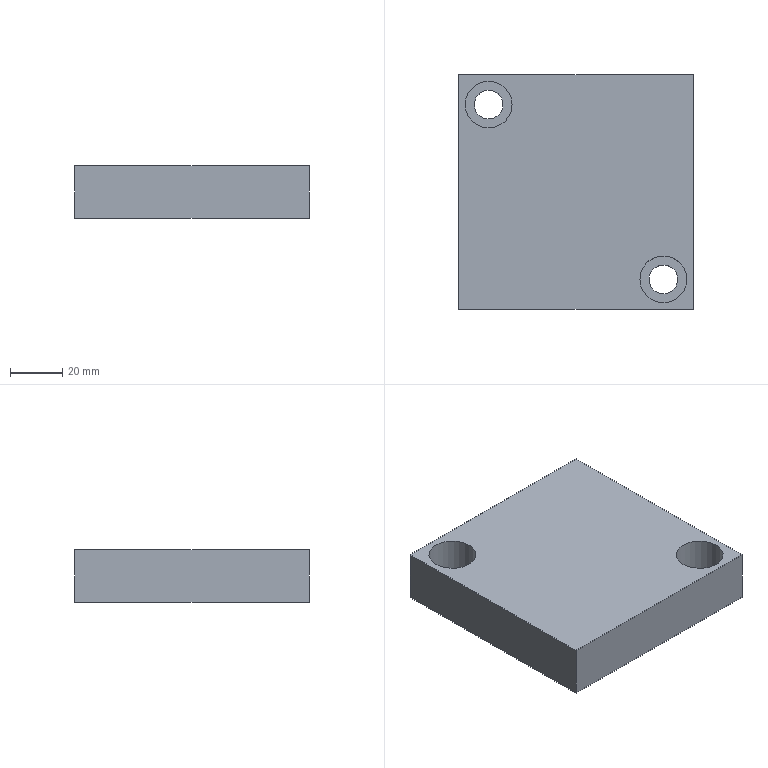Part | NX | features solid 2 | 1 solid | 12 faces | box 90 x 90 x 20 mm | volume 154053 mm3 | plane 8 | cylinder 4 | commonest cylinder face diameters 11 x2 18 x2
STEP:
#1=CARTESIAN_POINT('',(-2175.,-680.,-16.));
#2=VERTEX_POINT('',#1);
#3=CARTESIAN_POINT('',(-2175.,-680.,-36.));
#4=VERTEX_POINT('',#3);
#5=CARTESIAN_POINT('',(-2175.,-680.,-16.));
#6=DIRECTION('',(0.,0.,-1.));
#7=VECTOR('',#6,1000.);
#8=LINE('',#5,#7);
#9=EDGE_CURVE('',#2,#4,#8,.T.);
#10=ORIENTED_EDGE('',*,*,#9,.T.);
#11=CARTESIAN_POINT('',(-2085.,-680.,-36.));
#12=VERTEX_POINT('',#11);
#13=CARTESIAN_POINT('',(-2094.5,-680.,-36.));
#14=DIRECTION('',(-1.,0.,0.));
#15=VECTOR('',#14,1000.);
#16=LINE('',#13,#15);
#17=EDGE_CURVE('',#12,#4,#16,.T.);
#18=ORIENTED_EDGE('',*,*,#17,.F.);
#19=CARTESIAN_POINT('',(-2085.,-680.,-16.));
#20=VERTEX_POINT('',#19);
#21=CARTESIAN_POINT('',(-2085.,-680.,-16.));
#22=DIRECTION('',(0.,0.,1.));
#23=VECTOR('',#22,1000.);
#24=LINE('',#21,#23);
#25=EDGE_CURVE('',#20,#12,#24,.F.);
#26=ORIENTED_EDGE('',*,*,#25,.F.);
#27=CARTESIAN_POINT('',(-2094.5,-680.,-16.));
#28=DIRECTION('',(-1.,0.,0.));
#29=VECTOR('',#28,1000.);
#30=LINE('',#27,#29);
#31=EDGE_CURVE('',#20,#2,#30,.T.);
#32=ORIENTED_EDGE('',*,*,#31,.T.);
#33=EDGE_LOOP('',(#10,#18,#26,#32));
#34=FACE_BOUND('',#33,.T.);
#35=CARTESIAN_POINT('',(-2094.5,-680.,-16.));
#36=DIRECTION('',(0.,-1.,0.));
#37=DIRECTION('',(-1.,0.,0.));
#38=AXIS2_PLACEMENT_3D('',#35,#36,#37);
#39=PLANE('',#38);
#40=ADVANCED_FACE('',(#34),#39,.T.);
#41=ORIENTED_EDGE('',*,*,#25,.T.);
#42=CARTESIAN_POINT('',(-2085.,-590.,-36.));
#43=VERTEX_POINT('',#42);
#44=CARTESIAN_POINT('',(-2085.,-670.5,-36.));
#45=DIRECTION('',(0.,-1.,0.));
#46=VECTOR('',#45,1000.);
#47=LINE('',#44,#46);
#48=EDGE_CURVE('',#12,#43,#47,.F.);
#49=ORIENTED_EDGE('',*,*,#48,.T.);
#50=CARTESIAN_POINT('',(-2085.,-590.,-16.));
#51=VERTEX_POINT('',#50);
#52=CARTESIAN_POINT('',(-2085.,-590.,-16.));
#53=DIRECTION('',(0.,0.,-1.));
#54=VECTOR('',#53,1000.);
#55=LINE('',#52,#54);
#56=EDGE_CURVE('',#51,#43,#55,.T.);
#57=ORIENTED_EDGE('',*,*,#56,.F.);
#58=CARTESIAN_POINT('',(-2085.,-670.5,-16.));
#59=DIRECTION('',(0.,-1.,0.));
#60=VECTOR('',#59,1000.);
#61=LINE('',#58,#60);
#62=EDGE_CURVE('',#20,#51,#61,.F.);
#63=ORIENTED_EDGE('',*,*,#62,.F.);
#64=EDGE_LOOP('',(#41,#49,#57,#63));
#65=FACE_BOUND('',#64,.T.);
#66=CARTESIAN_POINT('',(-2085.,-670.5,-16.));
#67=DIRECTION('',(-1.,0.,0.));
#68=DIRECTION('',(0.,1.,0.));
#69=AXIS2_PLACEMENT_3D('',#66,#67,#68);
#70=PLANE('',#69);
#71=ADVANCED_FACE('',(#65),#70,.F.);
#72=ORIENTED_EDGE('',*,*,#56,.T.);
#73=CARTESIAN_POINT('',(-2175.,-590.,-36.));
#74=VERTEX_POINT('',#73);
#75=CARTESIAN_POINT('',(-2094.5,-590.,-36.));
#76=DIRECTION('',(1.,0.,0.));
#77=VECTOR('',#76,1000.);
#78=LINE('',#75,#77);
#79=EDGE_CURVE('',#43,#74,#78,.F.);
#80=ORIENTED_EDGE('',*,*,#79,.T.);
#81=CARTESIAN_POINT('',(-2175.,-590.,-16.));
#82=VERTEX_POINT('',#81);
#83=CARTESIAN_POINT('',(-2175.,-590.,-16.));
#84=DIRECTION('',(0.,0.,1.));
#85=VECTOR('',#84,1000.);
#86=LINE('',#83,#85);
#87=EDGE_CURVE('',#82,#74,#86,.F.);
#88=ORIENTED_EDGE('',*,*,#87,.F.);
#89=CARTESIAN_POINT('',(-2094.5,-590.,-16.));
#90=DIRECTION('',(1.,0.,0.));
#91=VECTOR('',#90,1000.);
#92=LINE('',#89,#91);
#93=EDGE_CURVE('',#51,#82,#92,.F.);
#94=ORIENTED_EDGE('',*,*,#93,.F.);
#95=EDGE_LOOP('',(#72,#80,#88,#94));
#96=FACE_BOUND('',#95,.T.);
#97=CARTESIAN_POINT('',(-2094.5,-590.,-16.));
#98=DIRECTION('',(0.,-1.,0.));
#99=DIRECTION('',(-1.,0.,0.));
#100=AXIS2_PLACEMENT_3D('',#97,#98,#99);
#101=PLANE('',#100);
#102=ADVANCED_FACE('',(#96),#101,.F.);
#103=CARTESIAN_POINT('',(-2175.,-670.5,-16.));
#104=DIRECTION('',(0.,1.,0.));
#105=VECTOR('',#104,1000.);
#106=LINE('',#103,#105);
#107=EDGE_CURVE('',#2,#82,#106,.T.);
#108=ORIENTED_EDGE('',*,*,#107,.T.);
#109=ORIENTED_EDGE('',*,*,#87,.T.);
#110=CARTESIAN_POINT('',(-2175.,-670.5,-36.));
#111=DIRECTION('',(0.,1.,0.));
#112=VECTOR('',#111,1000.);
#113=LINE('',#110,#112);
#114=EDGE_CURVE('',#4,#74,#113,.T.);
#115=ORIENTED_EDGE('',*,*,#114,.F.);
#116=ORIENTED_EDGE('',*,*,#9,.F.);
#117=EDGE_LOOP('',(#108,#109,#115,#116));
#118=FACE_BOUND('',#117,.T.);
#119=CARTESIAN_POINT('',(-2175.,-670.5,-16.));
#120=DIRECTION('',(-1.,0.,0.));
#121=DIRECTION('',(0.,1.,0.));
#122=AXIS2_PLACEMENT_3D('',#119,#120,#121);
#123=PLANE('',#122);
#124=ADVANCED_FACE('',(#118),#123,.T.);
#125=CARTESIAN_POINT('',(-2169.,-601.5,-36.));
#126=VERTEX_POINT('',#125);
#127=CARTESIAN_POINT('',(-2163.5,-601.5,-36.));
#128=DIRECTION('',(0.,0.,1.));
#129=DIRECTION('',(-1.,0.,0.));
#130=AXIS2_PLACEMENT_3D('',#127,#128,#129);
#131=CIRCLE('',#130,5.5);
#132=EDGE_CURVE('',#126,#126,#131,.T.);
#133=ORIENTED_EDGE('',*,*,#132,.T.);
#134=EDGE_LOOP('',(#133));
#135=FACE_BOUND('',#134,.T.);
#136=CARTESIAN_POINT('',(-2102.,-668.5,-36.));
#137=VERTEX_POINT('',#136);
#138=CARTESIAN_POINT('',(-2096.5,-668.5,-36.));
#139=DIRECTION('',(0.,0.,1.));
#140=DIRECTION('',(-1.,0.,0.));
#141=AXIS2_PLACEMENT_3D('',#138,#139,#140);
#142=CIRCLE('',#141,5.5);
#143=EDGE_CURVE('',#137,#137,#142,.T.);
#144=ORIENTED_EDGE('',*,*,#143,.T.);
#145=EDGE_LOOP('',(#144));
#146=FACE_BOUND('',#145,.T.);
#147=ORIENTED_EDGE('',*,*,#79,.F.);
#148=ORIENTED_EDGE('',*,*,#48,.F.);
#149=ORIENTED_EDGE('',*,*,#17,.T.);
#150=ORIENTED_EDGE('',*,*,#114,.T.);
#151=EDGE_LOOP('',(#147,#148,#149,#150));
#152=FACE_BOUND('',#151,.T.);
#153=CARTESIAN_POINT('',(-2094.5,-670.5,-36.));
#154=DIRECTION('',(0.,0.,1.));
#155=DIRECTION('',(1.,0.,0.));
#156=AXIS2_PLACEMENT_3D('',#153,#154,#155);
#157=PLANE('',#156);
#158=ADVANCED_FACE('',(#135,#146,#152),#157,.F.);
#159=CARTESIAN_POINT('',(-2172.5,-601.5,-16.));
#160=VERTEX_POINT('',#159);
#161=CARTESIAN_POINT('',(-2163.5,-601.5,-16.));
#162=DIRECTION('',(0.,0.,1.));
#163=DIRECTION('',(-1.,0.,0.));
#164=AXIS2_PLACEMENT_3D('',#161,#162,#163);
#165=CIRCLE('',#164,9.);
#166=EDGE_CURVE('',#160,#160,#165,.T.);
#167=ORIENTED_EDGE('',*,*,#166,.F.);
#168=EDGE_LOOP('',(#167));
#169=FACE_BOUND('',#168,.T.);
#170=CARTESIAN_POINT('',(-2105.5,-668.5,-16.));
#171=VERTEX_POINT('',#170);
#172=CARTESIAN_POINT('',(-2096.5,-668.5,-16.));
#173=DIRECTION('',(0.,0.,1.));
#174=DIRECTION('',(-1.,0.,0.));
#175=AXIS2_PLACEMENT_3D('',#172,#173,#174);
#176=CIRCLE('',#175,9.);
#177=EDGE_CURVE('',#171,#171,#176,.T.);
#178=ORIENTED_EDGE('',*,*,#177,.F.);
#179=EDGE_LOOP('',(#178));
#180=FACE_BOUND('',#179,.T.);
#181=ORIENTED_EDGE('',*,*,#93,.T.);
#182=ORIENTED_EDGE('',*,*,#107,.F.);
#183=ORIENTED_EDGE('',*,*,#31,.F.);
#184=ORIENTED_EDGE('',*,*,#62,.T.);
#185=EDGE_LOOP('',(#181,#182,#183,#184));
#186=FACE_BOUND('',#185,.T.);
#187=CARTESIAN_POINT('',(-2094.5,-670.5,-16.));
#188=DIRECTION('',(0.,0.,1.));
#189=DIRECTION('',(1.,0.,0.));
#190=AXIS2_PLACEMENT_3D('',#187,#188,#189);
#191=PLANE('',#190);
#192=ADVANCED_FACE('',(#169,#180,#186),#191,.T.);
#193=ORIENTED_EDGE('',*,*,#143,.F.);
#194=EDGE_LOOP('',(#193));
#195=FACE_BOUND('',#194,.T.);
#196=CARTESIAN_POINT('',(-2102.,-668.5,-29.));
#197=VERTEX_POINT('',#196);
#198=CARTESIAN_POINT('',(-2096.5,-668.5,-29.));
#199=DIRECTION('',(0.,0.,1.));
#200=DIRECTION('',(-1.,0.,0.));
#201=AXIS2_PLACEMENT_3D('',#198,#199,#200);
#202=CIRCLE('',#201,5.5);
#203=EDGE_CURVE('',#197,#197,#202,.T.);
#204=ORIENTED_EDGE('',*,*,#203,.T.);
#205=EDGE_LOOP('',(#204));
#206=FACE_BOUND('',#205,.T.);
#207=CARTESIAN_POINT('',(-2096.5,-668.5,-36.));
#208=DIRECTION('',(0.,0.,-1.));
#209=DIRECTION('',(-1.,0.,0.));
#210=AXIS2_PLACEMENT_3D('',#207,#208,#209);
#211=CYLINDRICAL_SURFACE('',#210,5.5);
#212=ADVANCED_FACE('',(#195,#206),#211,.F.);
#213=ORIENTED_EDGE('',*,*,#203,.F.);
#214=EDGE_LOOP('',(#213));
#215=FACE_BOUND('',#214,.T.);
#216=CARTESIAN_POINT('',(-2105.5,-668.5,-29.));
#217=VERTEX_POINT('',#216);
#218=CARTESIAN_POINT('',(-2096.5,-668.5,-29.));
#219=DIRECTION('',(0.,0.,1.));
#220=DIRECTION('',(-1.,0.,0.));
#221=AXIS2_PLACEMENT_3D('',#218,#219,#220);
#222=CIRCLE('',#221,9.);
#223=EDGE_CURVE('',#217,#217,#222,.T.);
#224=ORIENTED_EDGE('',*,*,#223,.T.);
#225=EDGE_LOOP('',(#224));
#226=FACE_BOUND('',#225,.T.);
#227=CARTESIAN_POINT('',(-2096.5,-668.5,-29.));
#228=DIRECTION('',(0.,0.,-1.));
#229=DIRECTION('',(-1.,0.,0.));
#230=AXIS2_PLACEMENT_3D('',#227,#228,#229);
#231=PLANE('',#230);
#232=ADVANCED_FACE('',(#215,#226),#231,.F.);
#233=ORIENTED_EDGE('',*,*,#223,.F.);
#234=EDGE_LOOP('',(#233));
#235=FACE_BOUND('',#234,.T.);
#236=ORIENTED_EDGE('',*,*,#177,.T.);
#237=EDGE_LOOP('',(#236));
#238=FACE_BOUND('',#237,.T.);
#239=CARTESIAN_POINT('',(-2096.5,-668.5,-16.));
#240=DIRECTION('',(0.,0.,-1.));
#241=DIRECTION('',(-1.,0.,0.));
#242=AXIS2_PLACEMENT_3D('',#239,#240,#241);
#243=CYLINDRICAL_SURFACE('',#242,9.);
#244=ADVANCED_FACE('',(#235,#238),#243,.F.);
#245=ORIENTED_EDGE('',*,*,#132,.F.);
#246=EDGE_LOOP('',(#245));
#247=FACE_BOUND('',#246,.T.);
#248=CARTESIAN_POINT('',(-2169.,-601.5,-29.));
#249=VERTEX_POINT('',#248);
#250=CARTESIAN_POINT('',(-2163.5,-601.5,-29.));
#251=DIRECTION('',(0.,0.,1.));
#252=DIRECTION('',(-1.,0.,0.));
#253=AXIS2_PLACEMENT_3D('',#250,#251,#252);
#254=CIRCLE('',#253,5.5);
#255=EDGE_CURVE('',#249,#249,#254,.T.);
#256=ORIENTED_EDGE('',*,*,#255,.T.);
#257=EDGE_LOOP('',(#256));
#258=FACE_BOUND('',#257,.T.);
#259=CARTESIAN_POINT('',(-2163.5,-601.5,-36.));
#260=DIRECTION('',(0.,0.,-1.));
#261=DIRECTION('',(-1.,0.,0.));
#262=AXIS2_PLACEMENT_3D('',#259,#260,#261);
#263=CYLINDRICAL_SURFACE('',#262,5.5);
#264=ADVANCED_FACE('',(#247,#258),#263,.F.);
#265=ORIENTED_EDGE('',*,*,#255,.F.);
#266=EDGE_LOOP('',(#265));
#267=FACE_BOUND('',#266,.T.);
#268=CARTESIAN_POINT('',(-2172.5,-601.5,-29.));
#269=VERTEX_POINT('',#268);
#270=CARTESIAN_POINT('',(-2163.5,-601.5,-29.));
#271=DIRECTION('',(0.,0.,1.));
#272=DIRECTION('',(-1.,0.,0.));
#273=AXIS2_PLACEMENT_3D('',#270,#271,#272);
#274=CIRCLE('',#273,9.);
#275=EDGE_CURVE('',#269,#269,#274,.T.);
#276=ORIENTED_EDGE('',*,*,#275,.T.);
#277=EDGE_LOOP('',(#276));
#278=FACE_BOUND('',#277,.T.);
#279=CARTESIAN_POINT('',(-2163.5,-601.5,-29.));
#280=DIRECTION('',(0.,0.,-1.));
#281=DIRECTION('',(-1.,0.,0.));
#282=AXIS2_PLACEMENT_3D('',#279,#280,#281);
#283=PLANE('',#282);
#284=ADVANCED_FACE('',(#267,#278),#283,.F.);
#285=ORIENTED_EDGE('',*,*,#275,.F.);
#286=EDGE_LOOP('',(#285));
#287=FACE_BOUND('',#286,.T.);
#288=ORIENTED_EDGE('',*,*,#166,.T.);
#289=EDGE_LOOP('',(#288));
#290=FACE_BOUND('',#289,.T.);
#291=CARTESIAN_POINT('',(-2163.5,-601.5,-16.));
#292=DIRECTION('',(0.,0.,-1.));
#293=DIRECTION('',(-1.,0.,0.));
#294=AXIS2_PLACEMENT_3D('',#291,#292,#293);
#295=CYLINDRICAL_SURFACE('',#294,9.);
#296=ADVANCED_FACE('',(#287,#290),#295,.F.);
#297=CLOSED_SHELL('',(#40,#71,#102,#124,#158,#192,#212,#232,#244,#264,#284,#296));
#298=MANIFOLD_SOLID_BREP('',#297);
#299=(LENGTH_UNIT()NAMED_UNIT(*)SI_UNIT(.MILLI.,.METRE.));
#300=UNCERTAINTY_MEASURE_WITH_UNIT(LENGTH_MEASURE(0.00001),#299,'','');
#301=(NAMED_UNIT(*)PLANE_ANGLE_UNIT()SI_UNIT($,.RADIAN.));
#302=(NAMED_UNIT(*)SI_UNIT($,.STERADIAN.)SOLID_ANGLE_UNIT());
#303=(GEOMETRIC_REPRESENTATION_CONTEXT(3)GLOBAL_UNCERTAINTY_ASSIGNED_CONTEXT((#300))GLOBAL_UNIT_ASSIGNED_CONTEXT((#299,#301,#302))REPRESENTATION_CONTEXT('',''));
#304=ADVANCED_BREP_SHAPE_REPRESENTATION('',(#298),#303);